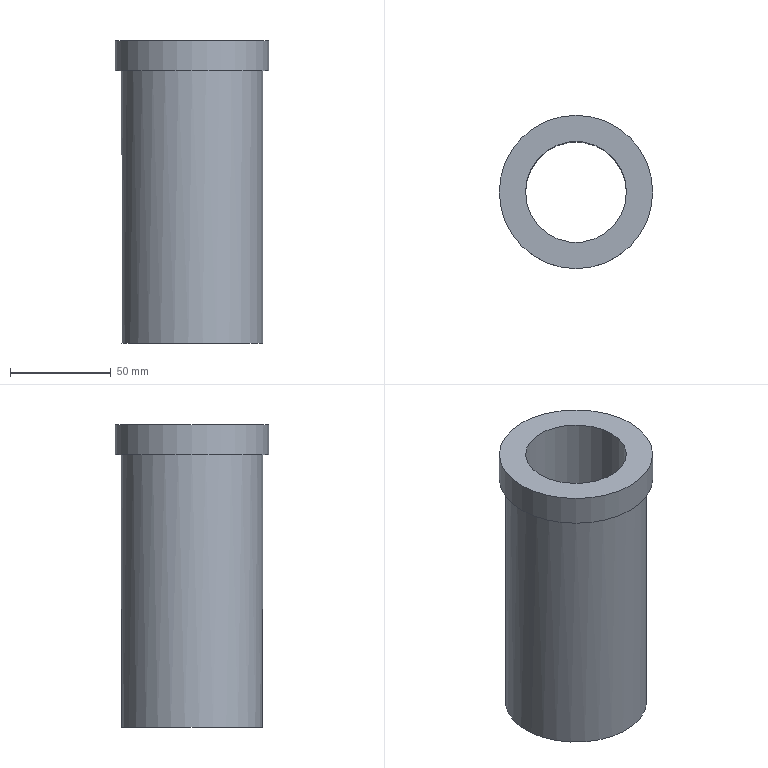Part | STEP file | GB-D50-150L | 1 solid | 6 faces | box 76 x 76 x 150 mm | volume 293063 mm3 | plane 3 | cylinder 3 | commonest cylinder face diameters 50 x1 70 x1 76 x1
STEP:
#1=CARTESIAN_POINT('',(0.,0.,0.));
#2=DIRECTION('',(0.,0.,1.));
#3=DIRECTION('',(1.,0.,0.));
#4=AXIS2_PLACEMENT_3D('',#1,#2,#3);
#5=CARTESIAN_POINT('',(260.,-270.,171.));
#6=VERTEX_POINT('',#5);
#7=CARTESIAN_POINT('',(222.,-270.,171.));
#8=DIRECTION('',(0.,0.,1.));
#9=DIRECTION('',(1.,0.,0.));
#10=AXIS2_PLACEMENT_3D('',#7,#8,#9);
#11=CIRCLE('',#10,38.);
#12=CARTESIAN_POINT('',(-165.,-340.,171.));
#13=DIRECTION('',(0.,0.,-1.));
#14=DIRECTION('',(0.,-1.,0.));
#15=AXIS2_PLACEMENT_3D('',#12,#13,#14);
#16=PLANE('',#15);
#17=CARTESIAN_POINT('',(-70.,-425.));
#18=CARTESIAN_POINT('',(-135.818,-425.));
#19=CARTESIAN_POINT('',(-102.909,-368.));
#20=CARTESIAN_POINT('',(-70.,-311.));
#21=CARTESIAN_POINT('',(-37.091,-368.));
#22=CARTESIAN_POINT('',(-4.182,-425.));
#23=CARTESIAN_POINT('',(-70.,-425.));
#24=(BOUNDED_CURVE()B_SPLINE_CURVE(2,(#17,#18,#19,#20,#21,#22,#23),.UNSPECIFIED.,.T.,.F.)B_SPLINE_CURVE_WITH_KNOTS((1,2,2,2,2,1),(-2.094,0.,2.094,4.189,6.283,8.378),.UNSPECIFIED.)CURVE()GEOMETRIC_REPRESENTATION_ITEM()RATIONAL_B_SPLINE_CURVE((1.,0.5,1.,0.5,1.,0.5,1.))REPRESENTATION_ITEM(''));
#25=(GEOMETRIC_REPRESENTATION_CONTEXT(2)PARAMETRIC_REPRESENTATION_CONTEXT()REPRESENTATION_CONTEXT('',''));
#26=DEFINITIONAL_REPRESENTATION('',(#24),#25);
#27=PCURVE('',#16,#26);
#28=CARTESIAN_POINT('',(222.,-270.,691.));
#29=DIRECTION('',(0.,0.,-1.));
#30=DIRECTION('',(1.,0.,0.));
#31=AXIS2_PLACEMENT_3D('',#28,#29,#30);
#32=CYLINDRICAL_SURFACE('',#31,38.);
#33=CARTESIAN_POINT('',(6.283,520.));
#34=DIRECTION('',(-1.,0.));
#35=VECTOR('',#34,1.);
#36=LINE('',#33,#35);
#37=(GEOMETRIC_REPRESENTATION_CONTEXT(2)PARAMETRIC_REPRESENTATION_CONTEXT()REPRESENTATION_CONTEXT('',''));
#38=DEFINITIONAL_REPRESENTATION('',(#36),#37);
#39=PCURVE('',#32,#38);
#40=SURFACE_CURVE('',#11,(#27,#39),.PCURVE_S1.);
#41=EDGE_CURVE('',#6,#6,#40,.T.);
#42=ORIENTED_EDGE('',*,*,#41,.T.);
#43=EDGE_LOOP('',(#42));
#44=FACE_BOUND('',#43,.T.);
#45=CARTESIAN_POINT('',(247.,-270.,171.));
#46=VERTEX_POINT('',#45);
#47=CARTESIAN_POINT('',(222.,-270.,171.));
#48=DIRECTION('',(0.,0.,-1.));
#49=DIRECTION('',(1.,0.,0.));
#50=AXIS2_PLACEMENT_3D('',#47,#48,#49);
#51=CIRCLE('',#50,25.);
#52=CARTESIAN_POINT('',(-70.,-387.));
#53=DIRECTION('',(0.,-1.));
#54=AXIS2_PLACEMENT_2D('',#52,#53);
#55=CIRCLE('',#54,25.);
#56=(GEOMETRIC_REPRESENTATION_CONTEXT(2)PARAMETRIC_REPRESENTATION_CONTEXT()REPRESENTATION_CONTEXT('',''));
#57=DEFINITIONAL_REPRESENTATION('',(#55),#56);
#58=PCURVE('',#16,#57);
#59=CARTESIAN_POINT('',(222.,-270.,539.));
#60=DIRECTION('',(0.,0.,-1.));
#61=DIRECTION('',(1.,0.,0.));
#62=AXIS2_PLACEMENT_3D('',#59,#60,#61);
#63=CYLINDRICAL_SURFACE('',#62,25.);
#64=CARTESIAN_POINT('',(0.,368.));
#65=DIRECTION('',(1.,0.));
#66=VECTOR('',#65,1.);
#67=LINE('',#64,#66);
#68=(GEOMETRIC_REPRESENTATION_CONTEXT(2)PARAMETRIC_REPRESENTATION_CONTEXT()REPRESENTATION_CONTEXT('',''));
#69=DEFINITIONAL_REPRESENTATION('',(#67),#68);
#70=PCURVE('',#63,#69);
#71=SURFACE_CURVE('',#51,(#58,#70),.PCURVE_S1.);
#72=EDGE_CURVE('',#46,#46,#71,.T.);
#73=ORIENTED_EDGE('',*,*,#72,.T.);
#74=EDGE_LOOP('',(#73));
#75=FACE_BOUND('',#74,.T.);
#76=ADVANCED_FACE('',(#44,#75),#16,.F.);
#77=CARTESIAN_POINT('',(257.,-270.,21.));
#78=VERTEX_POINT('',#77);
#79=CARTESIAN_POINT('',(222.,-270.,21.));
#80=DIRECTION('',(0.,0.,1.));
#81=DIRECTION('',(1.,0.,0.));
#82=AXIS2_PLACEMENT_3D('',#79,#80,#81);
#83=CIRCLE('',#82,35.);
#84=CARTESIAN_POINT('',(0.,-540.,21.));
#85=DIRECTION('',(0.,0.,1.));
#86=DIRECTION('',(-1.,0.,0.));
#87=AXIS2_PLACEMENT_3D('',#84,#85,#86);
#88=PLANE('',#87);
#89=CARTESIAN_POINT('',(-222.,-270.));
#90=DIRECTION('',(-1.,0.));
#91=AXIS2_PLACEMENT_2D('',#89,#90);
#92=CIRCLE('',#91,35.);
#93=(GEOMETRIC_REPRESENTATION_CONTEXT(2)PARAMETRIC_REPRESENTATION_CONTEXT()REPRESENTATION_CONTEXT('',''));
#94=DEFINITIONAL_REPRESENTATION('',(#92),#93);
#95=PCURVE('',#88,#94);
#96=CARTESIAN_POINT('',(222.,-270.,691.));
#97=DIRECTION('',(0.,0.,-1.));
#98=DIRECTION('',(1.,0.,0.));
#99=AXIS2_PLACEMENT_3D('',#96,#97,#98);
#100=CYLINDRICAL_SURFACE('',#99,35.);
#101=CARTESIAN_POINT('',(6.283,670.));
#102=DIRECTION('',(-1.,0.));
#103=VECTOR('',#102,1.);
#104=LINE('',#101,#103);
#105=(GEOMETRIC_REPRESENTATION_CONTEXT(2)PARAMETRIC_REPRESENTATION_CONTEXT()REPRESENTATION_CONTEXT('',''));
#106=DEFINITIONAL_REPRESENTATION('',(#104),#105);
#107=PCURVE('',#100,#106);
#108=SURFACE_CURVE('',#83,(#95,#107),.PCURVE_S1.);
#109=EDGE_CURVE('',#78,#78,#108,.T.);
#110=ORIENTED_EDGE('',*,*,#109,.F.);
#111=EDGE_LOOP('',(#110));
#112=FACE_BOUND('',#111,.T.);
#113=CARTESIAN_POINT('',(247.,-270.,21.));
#114=VERTEX_POINT('',#113);
#115=CARTESIAN_POINT('',(222.,-270.,21.));
#116=DIRECTION('',(0.,0.,-1.));
#117=DIRECTION('',(1.,0.,0.));
#118=AXIS2_PLACEMENT_3D('',#115,#116,#117);
#119=CIRCLE('',#118,25.);
#120=CARTESIAN_POINT('',(-247.,-270.));
#121=CARTESIAN_POINT('',(-247.,-226.699));
#122=CARTESIAN_POINT('',(-209.5,-248.349));
#123=CARTESIAN_POINT('',(-172.,-270.));
#124=CARTESIAN_POINT('',(-209.5,-291.651));
#125=CARTESIAN_POINT('',(-247.,-313.301));
#126=CARTESIAN_POINT('',(-247.,-270.));
#127=(BOUNDED_CURVE()B_SPLINE_CURVE(2,(#120,#121,#122,#123,#124,#125,#126),.UNSPECIFIED.,.T.,.F.)B_SPLINE_CURVE_WITH_KNOTS((1,2,2,2,2,1),(-2.094,0.,2.094,4.189,6.283,8.378),.UNSPECIFIED.)CURVE()GEOMETRIC_REPRESENTATION_ITEM()RATIONAL_B_SPLINE_CURVE((1.,0.5,1.,0.5,1.,0.5,1.))REPRESENTATION_ITEM(''));
#128=(GEOMETRIC_REPRESENTATION_CONTEXT(2)PARAMETRIC_REPRESENTATION_CONTEXT()REPRESENTATION_CONTEXT('',''));
#129=DEFINITIONAL_REPRESENTATION('',(#127),#128);
#130=PCURVE('',#88,#129);
#131=CARTESIAN_POINT('',(0.,518.));
#132=DIRECTION('',(1.,0.));
#133=VECTOR('',#132,1.);
#134=LINE('',#131,#133);
#135=(GEOMETRIC_REPRESENTATION_CONTEXT(2)PARAMETRIC_REPRESENTATION_CONTEXT()REPRESENTATION_CONTEXT('',''));
#136=DEFINITIONAL_REPRESENTATION('',(#134),#135);
#137=PCURVE('',#63,#136);
#138=SURFACE_CURVE('',#119,(#130,#137),.PCURVE_S1.);
#139=EDGE_CURVE('',#114,#114,#138,.T.);
#140=ORIENTED_EDGE('',*,*,#139,.F.);
#141=EDGE_LOOP('',(#140));
#142=FACE_BOUND('',#141,.T.);
#143=ADVANCED_FACE('',(#112,#142),#88,.F.);
#144=ORIENTED_EDGE('',*,*,#109,.T.);
#145=CARTESIAN_POINT('',(257.,-270.,156.));
#146=VERTEX_POINT('',#145);
#147=CARTESIAN_POINT('',(257.,-270.,156.));
#148=CARTESIAN_POINT('',(257.,-270.,21.));
#149=B_SPLINE_CURVE_WITH_KNOTS('',1,(#147,#148),.UNSPECIFIED.,.F.,.F.,(2,2),(535.,670.),.PIECEWISE_BEZIER_KNOTS.);
#150=CARTESIAN_POINT('',(0.,0.));
#151=DIRECTION('',(0.,1.));
#152=VECTOR('',#151,1.);
#153=LINE('',#150,#152);
#154=(GEOMETRIC_REPRESENTATION_CONTEXT(2)PARAMETRIC_REPRESENTATION_CONTEXT()REPRESENTATION_CONTEXT('',''));
#155=DEFINITIONAL_REPRESENTATION('',(#153),#154);
#156=PCURVE('',#100,#155);
#157=CARTESIAN_POINT('',(6.283,0.));
#158=DIRECTION('',(0.,1.));
#159=VECTOR('',#158,1.);
#160=LINE('',#157,#159);
#161=(GEOMETRIC_REPRESENTATION_CONTEXT(2)PARAMETRIC_REPRESENTATION_CONTEXT()REPRESENTATION_CONTEXT('',''));
#162=DEFINITIONAL_REPRESENTATION('',(#160),#161);
#163=PCURVE('',#100,#162);
#164=SEAM_CURVE('',#149,(#156,#163),.PCURVE_S1.);
#165=EDGE_CURVE('',#146,#78,#164,.T.);
#166=ORIENTED_EDGE('',*,*,#165,.F.);
#167=CARTESIAN_POINT('',(187.,-270.,156.));
#168=VERTEX_POINT('',#167);
#169=CARTESIAN_POINT('',(222.,-270.,156.));
#170=DIRECTION('',(0.,0.,1.));
#171=DIRECTION('',(-1.,0.,0.));
#172=AXIS2_PLACEMENT_3D('',#169,#170,#171);
#173=CIRCLE('',#172,35.);
#174=CARTESIAN_POINT('',(3.142,535.));
#175=DIRECTION('',(-1.,0.));
#176=VECTOR('',#175,1.);
#177=LINE('',#174,#176);
#178=(GEOMETRIC_REPRESENTATION_CONTEXT(2)PARAMETRIC_REPRESENTATION_CONTEXT()REPRESENTATION_CONTEXT('',''));
#179=DEFINITIONAL_REPRESENTATION('',(#177),#178);
#180=PCURVE('',#100,#179);
#181=CARTESIAN_POINT('',(0.,-540.,156.));
#182=DIRECTION('',(0.,0.,1.));
#183=DIRECTION('',(-1.,0.,0.));
#184=AXIS2_PLACEMENT_3D('',#181,#182,#183);
#185=PLANE('',#184);
#186=CARTESIAN_POINT('',(-222.,-270.));
#187=DIRECTION('',(1.,0.));
#188=AXIS2_PLACEMENT_2D('',#186,#187);
#189=CIRCLE('',#188,35.);
#190=(GEOMETRIC_REPRESENTATION_CONTEXT(2)PARAMETRIC_REPRESENTATION_CONTEXT()REPRESENTATION_CONTEXT('',''));
#191=DEFINITIONAL_REPRESENTATION('',(#189),#190);
#192=PCURVE('',#185,#191);
#193=SURFACE_CURVE('',#173,(#180,#192),.PCURVE_S1.);
#194=EDGE_CURVE('',#168,#146,#193,.T.);
#195=ORIENTED_EDGE('',*,*,#194,.F.);
#196=CARTESIAN_POINT('',(222.,-270.,156.));
#197=DIRECTION('',(0.,0.,1.));
#198=DIRECTION('',(-1.,0.,0.));
#199=AXIS2_PLACEMENT_3D('',#196,#197,#198);
#200=CIRCLE('',#199,35.);
#201=CARTESIAN_POINT('',(9.425,535.));
#202=DIRECTION('',(-1.,0.));
#203=VECTOR('',#202,1.);
#204=LINE('',#201,#203);
#205=(GEOMETRIC_REPRESENTATION_CONTEXT(2)PARAMETRIC_REPRESENTATION_CONTEXT()REPRESENTATION_CONTEXT('',''));
#206=DEFINITIONAL_REPRESENTATION('',(#204),#205);
#207=PCURVE('',#100,#206);
#208=CARTESIAN_POINT('',(-222.,-270.));
#209=DIRECTION('',(1.,0.));
#210=AXIS2_PLACEMENT_2D('',#208,#209);
#211=CIRCLE('',#210,35.);
#212=(GEOMETRIC_REPRESENTATION_CONTEXT(2)PARAMETRIC_REPRESENTATION_CONTEXT()REPRESENTATION_CONTEXT('',''));
#213=DEFINITIONAL_REPRESENTATION('',(#211),#212);
#214=PCURVE('',#185,#213);
#215=SURFACE_CURVE('',#200,(#207,#214),.PCURVE_S1.);
#216=EDGE_CURVE('',#146,#168,#215,.T.);
#217=ORIENTED_EDGE('',*,*,#216,.F.);
#218=ORIENTED_EDGE('',*,*,#165,.T.);
#219=EDGE_LOOP('',(#144,#166,#195,#217,#218));
#220=FACE_BOUND('',#219,.T.);
#221=ADVANCED_FACE('',(#220),#100,.T.);
#222=CARTESIAN_POINT('',(184.,-270.,156.));
#223=VERTEX_POINT('',#222);
#224=CARTESIAN_POINT('',(260.,-270.,156.));
#225=VERTEX_POINT('',#224);
#226=CARTESIAN_POINT('',(222.,-270.,156.));
#227=DIRECTION('',(0.,0.,1.));
#228=DIRECTION('',(-1.,0.,0.));
#229=AXIS2_PLACEMENT_3D('',#226,#227,#228);
#230=CIRCLE('',#229,38.);
#231=CARTESIAN_POINT('',(3.142,535.));
#232=DIRECTION('',(-1.,0.));
#233=VECTOR('',#232,1.);
#234=LINE('',#231,#233);
#235=(GEOMETRIC_REPRESENTATION_CONTEXT(2)PARAMETRIC_REPRESENTATION_CONTEXT()REPRESENTATION_CONTEXT('',''));
#236=DEFINITIONAL_REPRESENTATION('',(#234),#235);
#237=PCURVE('',#32,#236);
#238=CARTESIAN_POINT('',(-222.,-270.));
#239=DIRECTION('',(1.,0.));
#240=AXIS2_PLACEMENT_2D('',#238,#239);
#241=CIRCLE('',#240,38.);
#242=(GEOMETRIC_REPRESENTATION_CONTEXT(2)PARAMETRIC_REPRESENTATION_CONTEXT()REPRESENTATION_CONTEXT('',''));
#243=DEFINITIONAL_REPRESENTATION('',(#241),#242);
#244=PCURVE('',#185,#243);
#245=SURFACE_CURVE('',#230,(#237,#244),.PCURVE_S1.);
#246=EDGE_CURVE('',#223,#225,#245,.T.);
#247=ORIENTED_EDGE('',*,*,#246,.T.);
#248=CARTESIAN_POINT('',(260.,-270.,171.));
#249=CARTESIAN_POINT('',(260.,-270.,156.));
#250=B_SPLINE_CURVE_WITH_KNOTS('',1,(#248,#249),.UNSPECIFIED.,.F.,.F.,(2,2),(520.,535.),.PIECEWISE_BEZIER_KNOTS.);
#251=CARTESIAN_POINT('',(0.,0.));
#252=DIRECTION('',(0.,1.));
#253=VECTOR('',#252,1.);
#254=LINE('',#251,#253);
#255=(GEOMETRIC_REPRESENTATION_CONTEXT(2)PARAMETRIC_REPRESENTATION_CONTEXT()REPRESENTATION_CONTEXT('',''));
#256=DEFINITIONAL_REPRESENTATION('',(#254),#255);
#257=PCURVE('',#32,#256);
#258=CARTESIAN_POINT('',(6.283,0.));
#259=DIRECTION('',(0.,1.));
#260=VECTOR('',#259,1.);
#261=LINE('',#258,#260);
#262=(GEOMETRIC_REPRESENTATION_CONTEXT(2)PARAMETRIC_REPRESENTATION_CONTEXT()REPRESENTATION_CONTEXT('',''));
#263=DEFINITIONAL_REPRESENTATION('',(#261),#262);
#264=PCURVE('',#32,#263);
#265=SEAM_CURVE('',#250,(#257,#264),.PCURVE_S1.);
#266=EDGE_CURVE('',#6,#225,#265,.T.);
#267=ORIENTED_EDGE('',*,*,#266,.F.);
#268=ORIENTED_EDGE('',*,*,#41,.F.);
#269=ORIENTED_EDGE('',*,*,#266,.T.);
#270=CARTESIAN_POINT('',(222.,-270.,156.));
#271=DIRECTION('',(0.,0.,1.));
#272=DIRECTION('',(-1.,0.,0.));
#273=AXIS2_PLACEMENT_3D('',#270,#271,#272);
#274=CIRCLE('',#273,38.);
#275=CARTESIAN_POINT('',(9.425,535.));
#276=DIRECTION('',(-1.,0.));
#277=VECTOR('',#276,1.);
#278=LINE('',#275,#277);
#279=(GEOMETRIC_REPRESENTATION_CONTEXT(2)PARAMETRIC_REPRESENTATION_CONTEXT()REPRESENTATION_CONTEXT('',''));
#280=DEFINITIONAL_REPRESENTATION('',(#278),#279);
#281=PCURVE('',#32,#280);
#282=CARTESIAN_POINT('',(-222.,-270.));
#283=DIRECTION('',(1.,0.));
#284=AXIS2_PLACEMENT_2D('',#282,#283);
#285=CIRCLE('',#284,38.);
#286=(GEOMETRIC_REPRESENTATION_CONTEXT(2)PARAMETRIC_REPRESENTATION_CONTEXT()REPRESENTATION_CONTEXT('',''));
#287=DEFINITIONAL_REPRESENTATION('',(#285),#286);
#288=PCURVE('',#185,#287);
#289=SURFACE_CURVE('',#274,(#281,#288),.PCURVE_S1.);
#290=EDGE_CURVE('',#225,#223,#289,.T.);
#291=ORIENTED_EDGE('',*,*,#290,.T.);
#292=EDGE_LOOP('',(#247,#267,#268,#269,#291));
#293=FACE_BOUND('',#292,.T.);
#294=ADVANCED_FACE('',(#293),#32,.T.);
#295=ORIENTED_EDGE('',*,*,#194,.T.);
#296=ORIENTED_EDGE('',*,*,#216,.T.);
#297=EDGE_LOOP('',(#295,#296));
#298=FACE_BOUND('',#297,.T.);
#299=ORIENTED_EDGE('',*,*,#246,.F.);
#300=ORIENTED_EDGE('',*,*,#290,.F.);
#301=EDGE_LOOP('',(#299,#300));
#302=FACE_BOUND('',#301,.T.);
#303=ADVANCED_FACE('',(#298,#302),#185,.F.);
#304=ORIENTED_EDGE('',*,*,#139,.F.);
#305=CARTESIAN_POINT('',(247.,-270.,171.));
#306=CARTESIAN_POINT('',(247.,-270.,21.));
#307=B_SPLINE_CURVE_WITH_KNOTS('',1,(#305,#306),.UNSPECIFIED.,.F.,.F.,(2,2),(368.,518.),.PIECEWISE_BEZIER_KNOTS.);
#308=CARTESIAN_POINT('',(0.,0.));
#309=DIRECTION('',(0.,1.));
#310=VECTOR('',#309,1.);
#311=LINE('',#308,#310);
#312=(GEOMETRIC_REPRESENTATION_CONTEXT(2)PARAMETRIC_REPRESENTATION_CONTEXT()REPRESENTATION_CONTEXT('',''));
#313=DEFINITIONAL_REPRESENTATION('',(#311),#312);
#314=PCURVE('',#63,#313);
#315=CARTESIAN_POINT('',(6.283,0.));
#316=DIRECTION('',(0.,1.));
#317=VECTOR('',#316,1.);
#318=LINE('',#315,#317);
#319=(GEOMETRIC_REPRESENTATION_CONTEXT(2)PARAMETRIC_REPRESENTATION_CONTEXT()REPRESENTATION_CONTEXT('',''));
#320=DEFINITIONAL_REPRESENTATION('',(#318),#319);
#321=PCURVE('',#63,#320);
#322=SEAM_CURVE('',#307,(#314,#321),.PCURVE_S1.);
#323=EDGE_CURVE('',#46,#114,#322,.T.);
#324=ORIENTED_EDGE('',*,*,#323,.F.);
#325=ORIENTED_EDGE('',*,*,#72,.T.);
#326=ORIENTED_EDGE('',*,*,#323,.T.);
#327=EDGE_LOOP('',(#304,#324,#325,#326));
#328=FACE_BOUND('',#327,.F.);
#329=ADVANCED_FACE('',(#328),#63,.F.);
#330=CLOSED_SHELL('',(#76,#143,#221,#294,#303,#329));
#331=MANIFOLD_SOLID_BREP('',#330);
#332=(LENGTH_UNIT()NAMED_UNIT(*)SI_UNIT(.MILLI.,.METRE.));
#333=UNCERTAINTY_MEASURE_WITH_UNIT(LENGTH_MEASURE(0.000005),#332,'','');
#334=(NAMED_UNIT(*)PLANE_ANGLE_UNIT()SI_UNIT($,.RADIAN.));
#335=(NAMED_UNIT(*)SI_UNIT($,.STERADIAN.)SOLID_ANGLE_UNIT());
#336=(GEOMETRIC_REPRESENTATION_CONTEXT(3)GLOBAL_UNCERTAINTY_ASSIGNED_CONTEXT((#333))GLOBAL_UNIT_ASSIGNED_CONTEXT((#332,#334,#335))REPRESENTATION_CONTEXT('',''));
#337=ADVANCED_BREP_SHAPE_REPRESENTATION('',(#4,#331),#336);